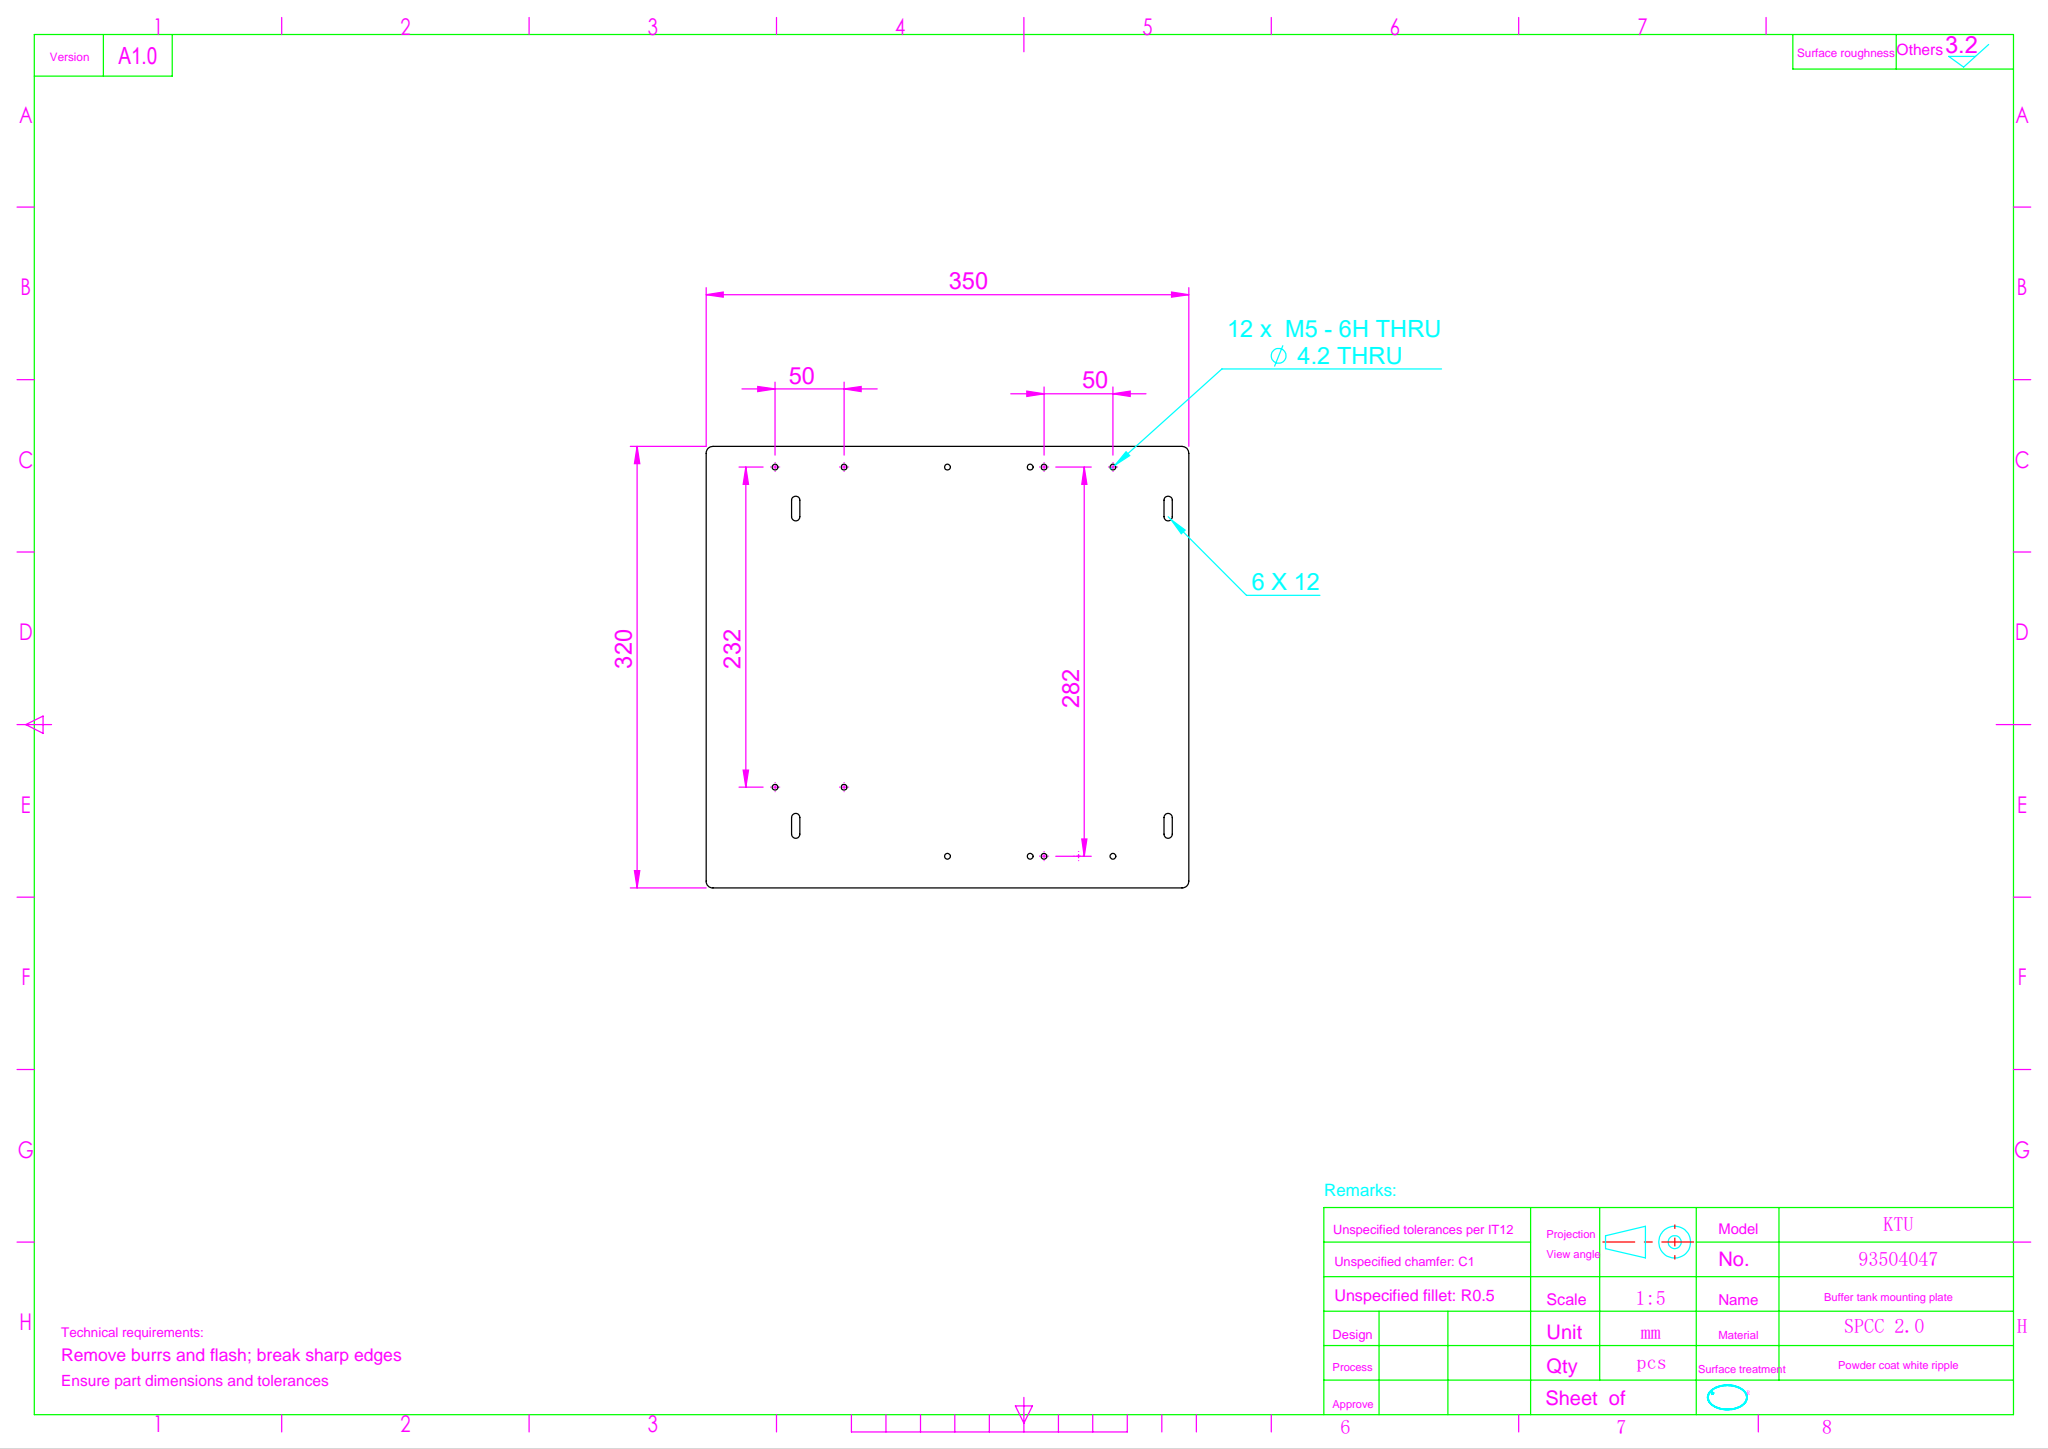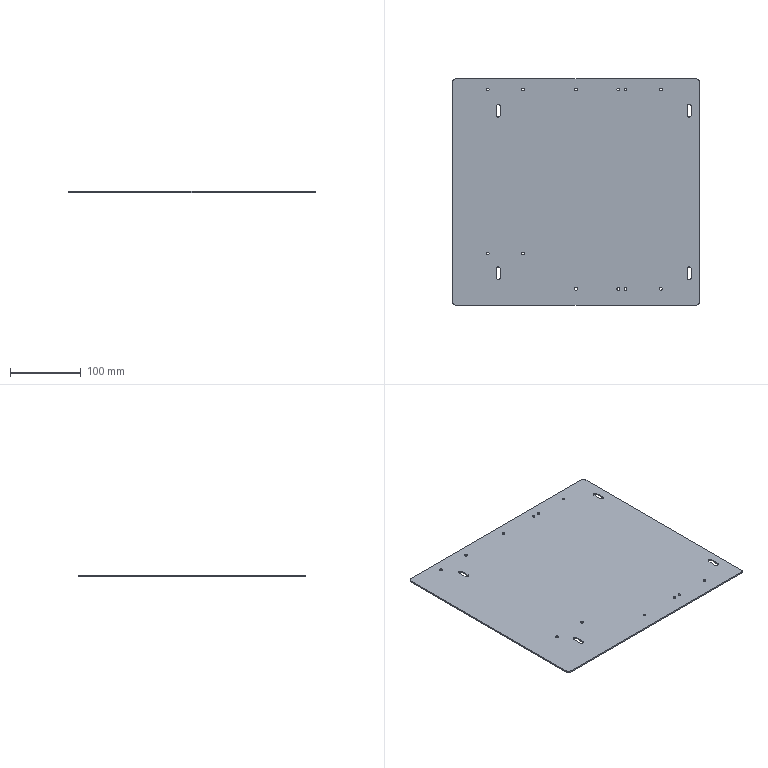Part | SolidWorks | features Fillet 1, FlatPattern 1, HoleWzd 1, ICE 1, LPattern 1, SMBaseFlange 1, SheetMetal 1 | 1 solid | 50 faces | box 350 x 320 x 2 mm | volume 222822 mm3 | cylinder 36 | plane 14 | commonest cylinder face diameters 4.2 x24 6 x8 10 x4